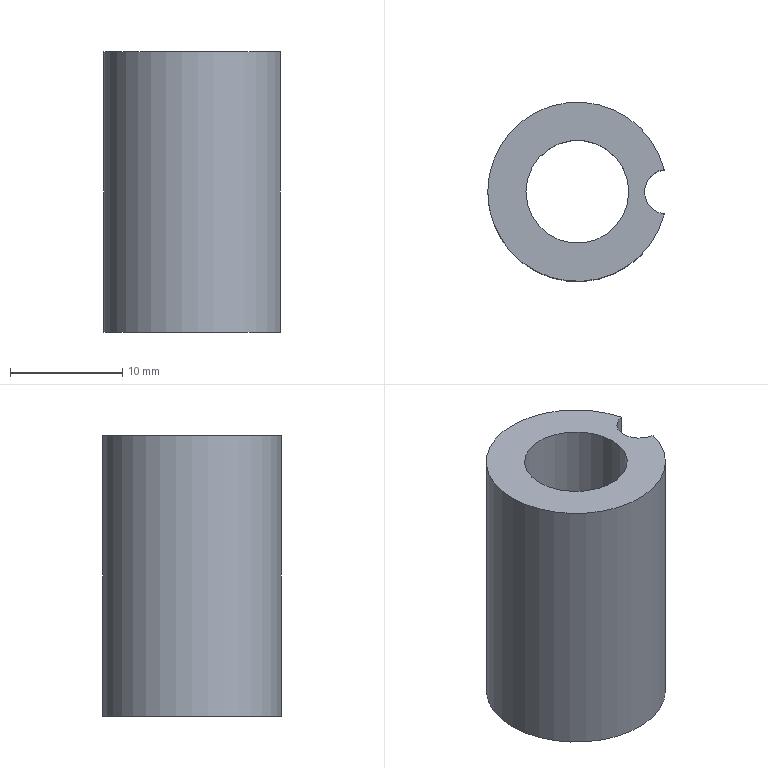Part | NX | features solid 2 | 1 solid | 7 faces | box 15.75 x 16 x 25 mm | volume 2848 mm3 | cylinder 4 | plane 3 | commonest cylinder face diameters 4 x1 9.18 x1 10.6 x1 16 x1
STEP:
#1=CARTESIAN_POINT('',(-507.846,-160.118,-12.396));
#2=VERTEX_POINT('',#1);
#3=CARTESIAN_POINT('',(-507.846,-164.087,-12.396));
#4=VERTEX_POINT('',#3);
#5=CARTESIAN_POINT('',(-507.596,-162.103,-12.396));
#6=DIRECTION('',(0.,0.,1.));
#7=DIRECTION('',(1.,0.,0.));
#8=AXIS2_PLACEMENT_3D('',#5,#6,#7);
#9=CIRCLE('',#8,2.);
#10=EDGE_CURVE('',#2,#4,#9,.T.);
#11=ORIENTED_EDGE('',*,*,#10,.F.);
#12=CARTESIAN_POINT('',(-515.596,-162.103,-12.396));
#13=DIRECTION('',(0.,0.,1.));
#14=DIRECTION('',(1.,0.,0.));
#15=AXIS2_PLACEMENT_3D('',#12,#13,#14);
#16=CIRCLE('',#15,8.);
#17=EDGE_CURVE('',#4,#2,#16,.F.);
#18=ORIENTED_EDGE('',*,*,#17,.F.);
#19=EDGE_LOOP('',(#11,#18));
#20=FACE_BOUND('',#19,.T.);
#21=CARTESIAN_POINT('',(-520.186,-162.103,-12.396));
#22=VERTEX_POINT('',#21);
#23=CARTESIAN_POINT('',(-515.596,-162.103,-12.396));
#24=DIRECTION('',(0.,0.,-1.));
#25=DIRECTION('',(-1.,0.,0.));
#26=AXIS2_PLACEMENT_3D('',#23,#24,#25);
#27=CIRCLE('',#26,4.59);
#28=EDGE_CURVE('',#22,#22,#27,.T.);
#29=ORIENTED_EDGE('',*,*,#28,.T.);
#30=EDGE_LOOP('',(#29));
#31=FACE_BOUND('',#30,.T.);
#32=CARTESIAN_POINT('',(-515.596,-162.103,-12.396));
#33=DIRECTION('',(0.,0.,1.));
#34=DIRECTION('',(1.,0.,0.));
#35=AXIS2_PLACEMENT_3D('',#32,#33,#34);
#36=PLANE('',#35);
#37=ADVANCED_FACE('',(#20,#31),#36,.T.);
#38=CARTESIAN_POINT('',(-507.846,-160.118,-37.396));
#39=VERTEX_POINT('',#38);
#40=CARTESIAN_POINT('',(-507.846,-164.087,-37.396));
#41=VERTEX_POINT('',#40);
#42=CARTESIAN_POINT('',(-507.596,-162.103,-37.396));
#43=DIRECTION('',(0.,0.,1.));
#44=DIRECTION('',(1.,0.,0.));
#45=AXIS2_PLACEMENT_3D('',#42,#43,#44);
#46=CIRCLE('',#45,2.);
#47=EDGE_CURVE('',#39,#41,#46,.T.);
#48=ORIENTED_EDGE('',*,*,#47,.T.);
#49=CARTESIAN_POINT('',(-515.596,-162.103,-37.396));
#50=DIRECTION('',(0.,0.,-1.));
#51=DIRECTION('',(-1.,0.,0.));
#52=AXIS2_PLACEMENT_3D('',#49,#50,#51);
#53=CIRCLE('',#52,8.);
#54=EDGE_CURVE('',#39,#41,#53,.F.);
#55=ORIENTED_EDGE('',*,*,#54,.F.);
#56=EDGE_LOOP('',(#48,#55));
#57=FACE_BOUND('',#56,.T.);
#58=CARTESIAN_POINT('',(-520.896,-162.103,-37.396));
#59=VERTEX_POINT('',#58);
#60=CARTESIAN_POINT('',(-515.596,-162.103,-37.396));
#61=DIRECTION('',(0.,0.,-1.));
#62=DIRECTION('',(-1.,0.,0.));
#63=AXIS2_PLACEMENT_3D('',#60,#61,#62);
#64=CIRCLE('',#63,5.3);
#65=EDGE_CURVE('',#59,#59,#64,.F.);
#66=ORIENTED_EDGE('',*,*,#65,.T.);
#67=EDGE_LOOP('',(#66));
#68=FACE_BOUND('',#67,.T.);
#69=CARTESIAN_POINT('',(-515.596,-162.103,-37.396));
#70=DIRECTION('',(0.,0.,-1.));
#71=DIRECTION('',(-1.,0.,0.));
#72=AXIS2_PLACEMENT_3D('',#69,#70,#71);
#73=PLANE('',#72);
#74=ADVANCED_FACE('',(#57,#68),#73,.T.);
#75=CARTESIAN_POINT('',(-507.846,-160.118,-24.896));
#76=DIRECTION('',(0.,0.,1.));
#77=VECTOR('',#76,1000.);
#78=LINE('',#75,#77);
#79=EDGE_CURVE('',#39,#2,#78,.T.);
#80=ORIENTED_EDGE('',*,*,#79,.F.);
#81=ORIENTED_EDGE('',*,*,#54,.T.);
#82=CARTESIAN_POINT('',(-507.846,-164.087,-24.896));
#83=DIRECTION('',(0.,0.,1.));
#84=VECTOR('',#83,1000.);
#85=LINE('',#82,#84);
#86=EDGE_CURVE('',#4,#41,#85,.F.);
#87=ORIENTED_EDGE('',*,*,#86,.F.);
#88=ORIENTED_EDGE('',*,*,#17,.T.);
#89=EDGE_LOOP('',(#80,#81,#87,#88));
#90=FACE_BOUND('',#89,.T.);
#91=CARTESIAN_POINT('',(-515.596,-162.103,-37.396));
#92=DIRECTION('',(0.,0.,1.));
#93=DIRECTION('',(1.,0.,0.));
#94=AXIS2_PLACEMENT_3D('',#91,#92,#93);
#95=CYLINDRICAL_SURFACE('',#94,8.);
#96=ADVANCED_FACE('',(#90),#95,.T.);
#97=CARTESIAN_POINT('',(-511.006,-162.103,-20.396));
#98=VERTEX_POINT('',#97);
#99=CARTESIAN_POINT('',(-515.596,-162.103,-20.396));
#100=DIRECTION('',(0.,0.,1.));
#101=DIRECTION('',(1.,0.,0.));
#102=AXIS2_PLACEMENT_3D('',#99,#100,#101);
#103=CIRCLE('',#102,4.59);
#104=EDGE_CURVE('',#98,#98,#103,.T.);
#105=ORIENTED_EDGE('',*,*,#104,.T.);
#106=EDGE_LOOP('',(#105));
#107=FACE_BOUND('',#106,.T.);
#108=CARTESIAN_POINT('',(-510.296,-162.103,-20.396));
#109=VERTEX_POINT('',#108);
#110=CARTESIAN_POINT('',(-515.596,-162.103,-20.396));
#111=DIRECTION('',(0.,0.,1.));
#112=DIRECTION('',(1.,0.,0.));
#113=AXIS2_PLACEMENT_3D('',#110,#111,#112);
#114=CIRCLE('',#113,5.3);
#115=EDGE_CURVE('',#109,#109,#114,.F.);
#116=ORIENTED_EDGE('',*,*,#115,.T.);
#117=EDGE_LOOP('',(#116));
#118=FACE_BOUND('',#117,.T.);
#119=CARTESIAN_POINT('',(-515.596,-162.103,-20.396));
#120=DIRECTION('',(0.,0.,1.));
#121=DIRECTION('',(1.,0.,0.));
#122=AXIS2_PLACEMENT_3D('',#119,#120,#121);
#123=PLANE('',#122);
#124=ADVANCED_FACE('',(#107,#118),#123,.F.);
#125=ORIENTED_EDGE('',*,*,#115,.F.);
#126=EDGE_LOOP('',(#125));
#127=FACE_BOUND('',#126,.T.);
#128=ORIENTED_EDGE('',*,*,#65,.F.);
#129=EDGE_LOOP('',(#128));
#130=FACE_BOUND('',#129,.T.);
#131=CARTESIAN_POINT('',(-515.596,-162.103,-37.396));
#132=DIRECTION('',(0.,0.,1.));
#133=DIRECTION('',(1.,0.,0.));
#134=AXIS2_PLACEMENT_3D('',#131,#132,#133);
#135=CYLINDRICAL_SURFACE('',#134,5.3);
#136=ADVANCED_FACE('',(#127,#130),#135,.F.);
#137=ORIENTED_EDGE('',*,*,#28,.F.);
#138=EDGE_LOOP('',(#137));
#139=FACE_BOUND('',#138,.T.);
#140=ORIENTED_EDGE('',*,*,#104,.F.);
#141=EDGE_LOOP('',(#140));
#142=FACE_BOUND('',#141,.T.);
#143=CARTESIAN_POINT('',(-515.596,-162.103,-20.396));
#144=DIRECTION('',(0.,0.,1.));
#145=DIRECTION('',(1.,0.,0.));
#146=AXIS2_PLACEMENT_3D('',#143,#144,#145);
#147=CYLINDRICAL_SURFACE('',#146,4.59);
#148=ADVANCED_FACE('',(#139,#142),#147,.F.);
#149=ORIENTED_EDGE('',*,*,#79,.T.);
#150=ORIENTED_EDGE('',*,*,#10,.T.);
#151=ORIENTED_EDGE('',*,*,#86,.T.);
#152=ORIENTED_EDGE('',*,*,#47,.F.);
#153=EDGE_LOOP('',(#149,#150,#151,#152));
#154=FACE_BOUND('',#153,.T.);
#155=CARTESIAN_POINT('',(-507.596,-162.103,-37.396));
#156=DIRECTION('',(0.,0.,1.));
#157=DIRECTION('',(1.,0.,0.));
#158=AXIS2_PLACEMENT_3D('',#155,#156,#157);
#159=CYLINDRICAL_SURFACE('',#158,2.);
#160=ADVANCED_FACE('',(#154),#159,.F.);
#161=CLOSED_SHELL('',(#37,#74,#96,#124,#136,#148,#160));
#162=MANIFOLD_SOLID_BREP('',#161);
#163=(LENGTH_UNIT()NAMED_UNIT(*)SI_UNIT(.MILLI.,.METRE.));
#164=UNCERTAINTY_MEASURE_WITH_UNIT(LENGTH_MEASURE(0.00001),#163,'','');
#165=(NAMED_UNIT(*)PLANE_ANGLE_UNIT()SI_UNIT($,.RADIAN.));
#166=(NAMED_UNIT(*)SI_UNIT($,.STERADIAN.)SOLID_ANGLE_UNIT());
#167=(GEOMETRIC_REPRESENTATION_CONTEXT(3)GLOBAL_UNCERTAINTY_ASSIGNED_CONTEXT((#164))GLOBAL_UNIT_ASSIGNED_CONTEXT((#163,#165,#166))REPRESENTATION_CONTEXT('',''));
#168=ADVANCED_BREP_SHAPE_REPRESENTATION('',(#162),#167);